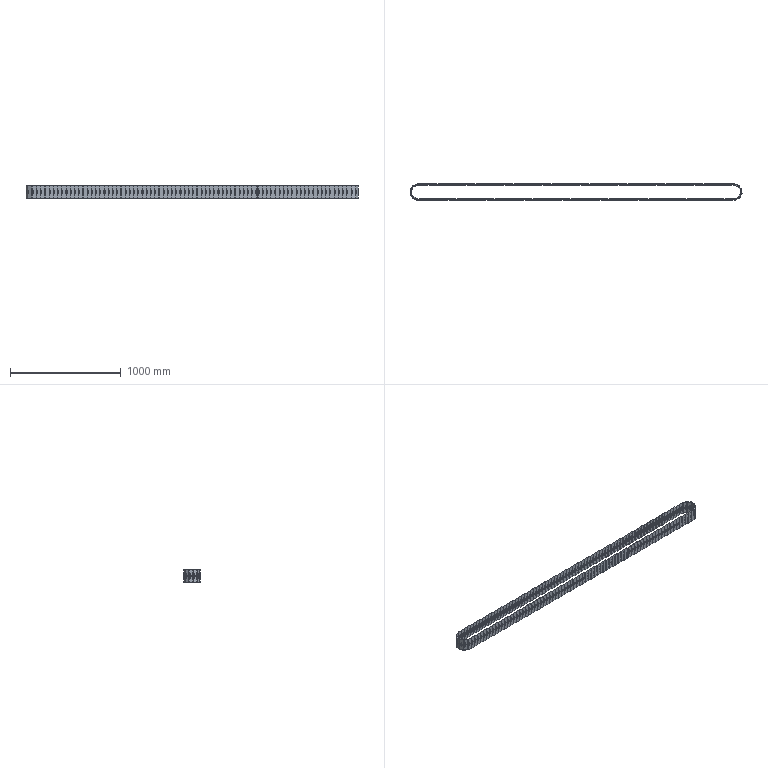Part | SolidWorks | 160 solids | 24960 faces | volume 3688939 mm3 | cylinder 12960 | plane 6720 | spline 5280 | commonest cylinder face diameters 1 x6400 12.8 x2080 4 x1600 6.36 x640 16.473 x480 17.088 x480